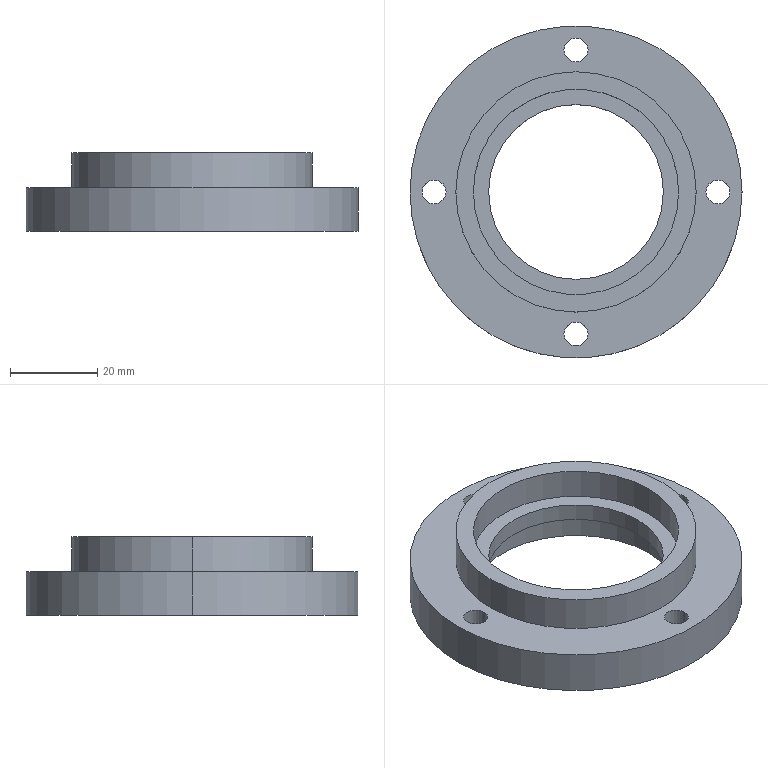Part | SolidWorks | features ICE 4, Extrusion 1, HoleWzd 1 | 1 solid | 35 faces | box 76 x 76 x 18 mm | volume 32922 mm3 | cylinder 26 | plane 9 | commonest cylinder face diameters 5.5 x8 10 x8 47 x4 40 x2 55 x2 76 x2
STEP:
#1=CARTESIAN_POINT('',(5.,32.5,5.4));
#2=VERTEX_POINT('',#1);
#3=CARTESIAN_POINT('',(-5.,32.5,5.4));
#4=VERTEX_POINT('',#3);
#5=CARTESIAN_POINT('',(0.,32.5,5.4));
#6=DIRECTION('',(0.,0.,-1.));
#7=DIRECTION('',(-1.,0.,0.));
#8=AXIS2_PLACEMENT_3D('',#5,#6,#7);
#9=CIRCLE('',#8,5.);
#10=EDGE_CURVE('',#2,#4,#9,.T.);
#11=ORIENTED_EDGE('',*,*,#10,.F.);
#12=CARTESIAN_POINT('',(5.,32.5,0.));
#13=VERTEX_POINT('',#12);
#14=CARTESIAN_POINT('',(5.,32.5,0.));
#15=DIRECTION('',(0.,0.,-1.));
#16=VECTOR('',#15,1000.);
#17=LINE('',#14,#16);
#18=EDGE_CURVE('',#2,#13,#17,.T.);
#19=ORIENTED_EDGE('',*,*,#18,.T.);
#20=CARTESIAN_POINT('',(-5.,32.5,0.));
#21=VERTEX_POINT('',#20);
#22=CARTESIAN_POINT('',(0.,32.5,0.));
#23=DIRECTION('',(0.,0.,-1.));
#24=DIRECTION('',(-1.,0.,0.));
#25=AXIS2_PLACEMENT_3D('',#22,#23,#24);
#26=CIRCLE('',#25,5.);
#27=EDGE_CURVE('',#13,#21,#26,.T.);
#28=ORIENTED_EDGE('',*,*,#27,.T.);
#29=CARTESIAN_POINT('',(-5.,32.5,0.));
#30=DIRECTION('',(0.,0.,-1.));
#31=VECTOR('',#30,1000.);
#32=LINE('',#29,#31);
#33=EDGE_CURVE('',#4,#21,#32,.T.);
#34=ORIENTED_EDGE('',*,*,#33,.F.);
#35=EDGE_LOOP('',(#11,#19,#28,#34));
#36=FACE_OUTER_BOUND('',#35,.T.);
#37=CARTESIAN_POINT('',(0.,32.5,0.));
#38=DIRECTION('',(0.,0.,-1.));
#39=DIRECTION('',(-1.,0.,0.));
#40=AXIS2_PLACEMENT_3D('',#37,#38,#39);
#41=CYLINDRICAL_SURFACE('',#40,5.);
#42=ADVANCED_FACE('',(#36),#41,.F.);
#43=CARTESIAN_POINT('',(-2.75,32.5,10.));
#44=VERTEX_POINT('',#43);
#45=CARTESIAN_POINT('',(2.75,32.5,10.));
#46=VERTEX_POINT('',#45);
#47=CARTESIAN_POINT('',(0.,32.5,10.));
#48=DIRECTION('',(0.,0.,1.));
#49=DIRECTION('',(1.,0.,0.));
#50=AXIS2_PLACEMENT_3D('',#47,#48,#49);
#51=CIRCLE('',#50,2.75);
#52=EDGE_CURVE('',#44,#46,#51,.T.);
#53=ORIENTED_EDGE('',*,*,#52,.T.);
#54=CARTESIAN_POINT('',(2.75,32.5,5.4));
#55=VERTEX_POINT('',#54);
#56=CARTESIAN_POINT('',(2.75,32.5,0.));
#57=DIRECTION('',(0.,0.,-1.));
#58=VECTOR('',#57,1000.);
#59=LINE('',#56,#58);
#60=EDGE_CURVE('',#46,#55,#59,.T.);
#61=ORIENTED_EDGE('',*,*,#60,.T.);
#62=CARTESIAN_POINT('',(-2.75,32.5,5.4));
#63=VERTEX_POINT('',#62);
#64=CARTESIAN_POINT('',(0.,32.5,5.4));
#65=DIRECTION('',(0.,0.,-1.));
#66=DIRECTION('',(-1.,0.,0.));
#67=AXIS2_PLACEMENT_3D('',#64,#65,#66);
#68=CIRCLE('',#67,2.75);
#69=EDGE_CURVE('',#55,#63,#68,.T.);
#70=ORIENTED_EDGE('',*,*,#69,.T.);
#71=CARTESIAN_POINT('',(-2.75,32.5,0.));
#72=DIRECTION('',(0.,0.,-1.));
#73=VECTOR('',#72,1000.);
#74=LINE('',#71,#73);
#75=EDGE_CURVE('',#44,#63,#74,.T.);
#76=ORIENTED_EDGE('',*,*,#75,.F.);
#77=EDGE_LOOP('',(#53,#61,#70,#76));
#78=FACE_OUTER_BOUND('',#77,.T.);
#79=CARTESIAN_POINT('',(0.,32.5,0.));
#80=DIRECTION('',(0.,0.,-1.));
#81=DIRECTION('',(-1.,0.,0.));
#82=AXIS2_PLACEMENT_3D('',#79,#80,#81);
#83=CYLINDRICAL_SURFACE('',#82,2.75);
#84=ADVANCED_FACE('',(#78),#83,.F.);
#85=CARTESIAN_POINT('',(37.5,0.,5.4));
#86=VERTEX_POINT('',#85);
#87=CARTESIAN_POINT('',(27.5,0.,5.4));
#88=VERTEX_POINT('',#87);
#89=CARTESIAN_POINT('',(32.5,0.,5.4));
#90=DIRECTION('',(0.,0.,-1.));
#91=DIRECTION('',(-1.,0.,0.));
#92=AXIS2_PLACEMENT_3D('',#89,#90,#91);
#93=CIRCLE('',#92,5.);
#94=EDGE_CURVE('',#86,#88,#93,.T.);
#95=ORIENTED_EDGE('',*,*,#94,.F.);
#96=CARTESIAN_POINT('',(37.5,0.,0.));
#97=VERTEX_POINT('',#96);
#98=CARTESIAN_POINT('',(37.5,0.,0.));
#99=DIRECTION('',(0.,0.,-1.));
#100=VECTOR('',#99,1000.);
#101=LINE('',#98,#100);
#102=EDGE_CURVE('',#86,#97,#101,.T.);
#103=ORIENTED_EDGE('',*,*,#102,.T.);
#104=CARTESIAN_POINT('',(27.5,0.,0.));
#105=VERTEX_POINT('',#104);
#106=CARTESIAN_POINT('',(32.5,0.,0.));
#107=DIRECTION('',(0.,0.,-1.));
#108=DIRECTION('',(-1.,0.,0.));
#109=AXIS2_PLACEMENT_3D('',#106,#107,#108);
#110=CIRCLE('',#109,5.);
#111=EDGE_CURVE('',#97,#105,#110,.T.);
#112=ORIENTED_EDGE('',*,*,#111,.T.);
#113=CARTESIAN_POINT('',(27.5,0.,0.));
#114=DIRECTION('',(0.,0.,-1.));
#115=VECTOR('',#114,1000.);
#116=LINE('',#113,#115);
#117=EDGE_CURVE('',#88,#105,#116,.T.);
#118=ORIENTED_EDGE('',*,*,#117,.F.);
#119=EDGE_LOOP('',(#95,#103,#112,#118));
#120=FACE_OUTER_BOUND('',#119,.T.);
#121=CARTESIAN_POINT('',(32.5,0.,0.));
#122=DIRECTION('',(0.,0.,-1.));
#123=DIRECTION('',(-1.,0.,0.));
#124=AXIS2_PLACEMENT_3D('',#121,#122,#123);
#125=CYLINDRICAL_SURFACE('',#124,5.);
#126=ADVANCED_FACE('',(#120),#125,.F.);
#127=CARTESIAN_POINT('',(29.75,0.,10.));
#128=VERTEX_POINT('',#127);
#129=CARTESIAN_POINT('',(35.25,0.,10.));
#130=VERTEX_POINT('',#129);
#131=CARTESIAN_POINT('',(32.5,0.,10.));
#132=DIRECTION('',(0.,0.,1.));
#133=DIRECTION('',(1.,0.,0.));
#134=AXIS2_PLACEMENT_3D('',#131,#132,#133);
#135=CIRCLE('',#134,2.75);
#136=EDGE_CURVE('',#128,#130,#135,.T.);
#137=ORIENTED_EDGE('',*,*,#136,.T.);
#138=CARTESIAN_POINT('',(35.25,0.,5.4));
#139=VERTEX_POINT('',#138);
#140=CARTESIAN_POINT('',(35.25,0.,0.));
#141=DIRECTION('',(0.,0.,-1.));
#142=VECTOR('',#141,1000.);
#143=LINE('',#140,#142);
#144=EDGE_CURVE('',#130,#139,#143,.T.);
#145=ORIENTED_EDGE('',*,*,#144,.T.);
#146=CARTESIAN_POINT('',(29.75,0.,5.4));
#147=VERTEX_POINT('',#146);
#148=CARTESIAN_POINT('',(32.5,0.,5.4));
#149=DIRECTION('',(0.,0.,-1.));
#150=DIRECTION('',(-1.,0.,0.));
#151=AXIS2_PLACEMENT_3D('',#148,#149,#150);
#152=CIRCLE('',#151,2.75);
#153=EDGE_CURVE('',#139,#147,#152,.T.);
#154=ORIENTED_EDGE('',*,*,#153,.T.);
#155=CARTESIAN_POINT('',(29.75,0.,0.));
#156=DIRECTION('',(0.,0.,-1.));
#157=VECTOR('',#156,1000.);
#158=LINE('',#155,#157);
#159=EDGE_CURVE('',#128,#147,#158,.T.);
#160=ORIENTED_EDGE('',*,*,#159,.F.);
#161=EDGE_LOOP('',(#137,#145,#154,#160));
#162=FACE_OUTER_BOUND('',#161,.T.);
#163=CARTESIAN_POINT('',(32.5,0.,0.));
#164=DIRECTION('',(0.,0.,-1.));
#165=DIRECTION('',(-1.,0.,0.));
#166=AXIS2_PLACEMENT_3D('',#163,#164,#165);
#167=CYLINDRICAL_SURFACE('',#166,2.75);
#168=ADVANCED_FACE('',(#162),#167,.F.);
#169=CARTESIAN_POINT('',(5.,-32.5,5.4));
#170=VERTEX_POINT('',#169);
#171=CARTESIAN_POINT('',(-5.,-32.5,5.4));
#172=VERTEX_POINT('',#171);
#173=CARTESIAN_POINT('',(0.,-32.5,5.4));
#174=DIRECTION('',(0.,0.,-1.));
#175=DIRECTION('',(-1.,0.,0.));
#176=AXIS2_PLACEMENT_3D('',#173,#174,#175);
#177=CIRCLE('',#176,5.);
#178=EDGE_CURVE('',#170,#172,#177,.T.);
#179=ORIENTED_EDGE('',*,*,#178,.F.);
#180=CARTESIAN_POINT('',(5.,-32.5,0.));
#181=VERTEX_POINT('',#180);
#182=CARTESIAN_POINT('',(5.,-32.5,0.));
#183=DIRECTION('',(0.,0.,-1.));
#184=VECTOR('',#183,1000.);
#185=LINE('',#182,#184);
#186=EDGE_CURVE('',#170,#181,#185,.T.);
#187=ORIENTED_EDGE('',*,*,#186,.T.);
#188=CARTESIAN_POINT('',(-5.,-32.5,0.));
#189=VERTEX_POINT('',#188);
#190=CARTESIAN_POINT('',(0.,-32.5,0.));
#191=DIRECTION('',(0.,0.,-1.));
#192=DIRECTION('',(-1.,0.,0.));
#193=AXIS2_PLACEMENT_3D('',#190,#191,#192);
#194=CIRCLE('',#193,5.);
#195=EDGE_CURVE('',#181,#189,#194,.T.);
#196=ORIENTED_EDGE('',*,*,#195,.T.);
#197=CARTESIAN_POINT('',(-5.,-32.5,0.));
#198=DIRECTION('',(0.,0.,-1.));
#199=VECTOR('',#198,1000.);
#200=LINE('',#197,#199);
#201=EDGE_CURVE('',#172,#189,#200,.T.);
#202=ORIENTED_EDGE('',*,*,#201,.F.);
#203=EDGE_LOOP('',(#179,#187,#196,#202));
#204=FACE_OUTER_BOUND('',#203,.T.);
#205=CARTESIAN_POINT('',(0.,-32.5,0.));
#206=DIRECTION('',(0.,0.,-1.));
#207=DIRECTION('',(-1.,0.,0.));
#208=AXIS2_PLACEMENT_3D('',#205,#206,#207);
#209=CYLINDRICAL_SURFACE('',#208,5.);
#210=ADVANCED_FACE('',(#204),#209,.F.);
#211=CARTESIAN_POINT('',(-2.75,-32.5,10.));
#212=VERTEX_POINT('',#211);
#213=CARTESIAN_POINT('',(2.75,-32.5,10.));
#214=VERTEX_POINT('',#213);
#215=CARTESIAN_POINT('',(0.,-32.5,10.));
#216=DIRECTION('',(0.,0.,1.));
#217=DIRECTION('',(1.,0.,0.));
#218=AXIS2_PLACEMENT_3D('',#215,#216,#217);
#219=CIRCLE('',#218,2.75);
#220=EDGE_CURVE('',#212,#214,#219,.T.);
#221=ORIENTED_EDGE('',*,*,#220,.T.);
#222=CARTESIAN_POINT('',(2.75,-32.5,5.4));
#223=VERTEX_POINT('',#222);
#224=CARTESIAN_POINT('',(2.75,-32.5,0.));
#225=DIRECTION('',(0.,0.,-1.));
#226=VECTOR('',#225,1000.);
#227=LINE('',#224,#226);
#228=EDGE_CURVE('',#214,#223,#227,.T.);
#229=ORIENTED_EDGE('',*,*,#228,.T.);
#230=CARTESIAN_POINT('',(-2.75,-32.5,5.4));
#231=VERTEX_POINT('',#230);
#232=CARTESIAN_POINT('',(0.,-32.5,5.4));
#233=DIRECTION('',(0.,0.,-1.));
#234=DIRECTION('',(-1.,0.,0.));
#235=AXIS2_PLACEMENT_3D('',#232,#233,#234);
#236=CIRCLE('',#235,2.75);
#237=EDGE_CURVE('',#223,#231,#236,.T.);
#238=ORIENTED_EDGE('',*,*,#237,.T.);
#239=CARTESIAN_POINT('',(-2.75,-32.5,0.));
#240=DIRECTION('',(0.,0.,-1.));
#241=VECTOR('',#240,1000.);
#242=LINE('',#239,#241);
#243=EDGE_CURVE('',#212,#231,#242,.T.);
#244=ORIENTED_EDGE('',*,*,#243,.F.);
#245=EDGE_LOOP('',(#221,#229,#238,#244));
#246=FACE_OUTER_BOUND('',#245,.T.);
#247=CARTESIAN_POINT('',(0.,-32.5,0.));
#248=DIRECTION('',(0.,0.,-1.));
#249=DIRECTION('',(-1.,0.,0.));
#250=AXIS2_PLACEMENT_3D('',#247,#248,#249);
#251=CYLINDRICAL_SURFACE('',#250,2.75);
#252=ADVANCED_FACE('',(#246),#251,.F.);
#253=CARTESIAN_POINT('',(-27.5,0.,5.4));
#254=VERTEX_POINT('',#253);
#255=CARTESIAN_POINT('',(-37.5,0.,5.4));
#256=VERTEX_POINT('',#255);
#257=CARTESIAN_POINT('',(-32.5,0.,5.4));
#258=DIRECTION('',(0.,0.,-1.));
#259=DIRECTION('',(-1.,0.,0.));
#260=AXIS2_PLACEMENT_3D('',#257,#258,#259);
#261=CIRCLE('',#260,5.);
#262=EDGE_CURVE('',#254,#256,#261,.T.);
#263=ORIENTED_EDGE('',*,*,#262,.F.);
#264=CARTESIAN_POINT('',(-27.5,0.,0.));
#265=VERTEX_POINT('',#264);
#266=CARTESIAN_POINT('',(-27.5,0.,0.));
#267=DIRECTION('',(0.,0.,-1.));
#268=VECTOR('',#267,1000.);
#269=LINE('',#266,#268);
#270=EDGE_CURVE('',#254,#265,#269,.T.);
#271=ORIENTED_EDGE('',*,*,#270,.T.);
#272=CARTESIAN_POINT('',(-37.5,0.,0.));
#273=VERTEX_POINT('',#272);
#274=CARTESIAN_POINT('',(-32.5,0.,0.));
#275=DIRECTION('',(0.,0.,-1.));
#276=DIRECTION('',(-1.,0.,0.));
#277=AXIS2_PLACEMENT_3D('',#274,#275,#276);
#278=CIRCLE('',#277,5.);
#279=EDGE_CURVE('',#265,#273,#278,.T.);
#280=ORIENTED_EDGE('',*,*,#279,.T.);
#281=CARTESIAN_POINT('',(-37.5,0.,0.));
#282=DIRECTION('',(0.,0.,-1.));
#283=VECTOR('',#282,1000.);
#284=LINE('',#281,#283);
#285=EDGE_CURVE('',#256,#273,#284,.T.);
#286=ORIENTED_EDGE('',*,*,#285,.F.);
#287=EDGE_LOOP('',(#263,#271,#280,#286));
#288=FACE_OUTER_BOUND('',#287,.T.);
#289=CARTESIAN_POINT('',(-32.5,0.,0.));
#290=DIRECTION('',(0.,0.,-1.));
#291=DIRECTION('',(-1.,0.,0.));
#292=AXIS2_PLACEMENT_3D('',#289,#290,#291);
#293=CYLINDRICAL_SURFACE('',#292,5.);
#294=ADVANCED_FACE('',(#288),#293,.F.);
#295=CARTESIAN_POINT('',(-35.25,0.,10.));
#296=VERTEX_POINT('',#295);
#297=CARTESIAN_POINT('',(-29.75,0.,10.));
#298=VERTEX_POINT('',#297);
#299=CARTESIAN_POINT('',(-32.5,0.,10.));
#300=DIRECTION('',(0.,0.,1.));
#301=DIRECTION('',(1.,0.,0.));
#302=AXIS2_PLACEMENT_3D('',#299,#300,#301);
#303=CIRCLE('',#302,2.75);
#304=EDGE_CURVE('',#296,#298,#303,.T.);
#305=ORIENTED_EDGE('',*,*,#304,.T.);
#306=CARTESIAN_POINT('',(-29.75,0.,5.4));
#307=VERTEX_POINT('',#306);
#308=CARTESIAN_POINT('',(-29.75,0.,0.));
#309=DIRECTION('',(0.,0.,-1.));
#310=VECTOR('',#309,1000.);
#311=LINE('',#308,#310);
#312=EDGE_CURVE('',#298,#307,#311,.T.);
#313=ORIENTED_EDGE('',*,*,#312,.T.);
#314=CARTESIAN_POINT('',(-35.25,0.,5.4));
#315=VERTEX_POINT('',#314);
#316=CARTESIAN_POINT('',(-32.5,0.,5.4));
#317=DIRECTION('',(0.,0.,-1.));
#318=DIRECTION('',(-1.,0.,0.));
#319=AXIS2_PLACEMENT_3D('',#316,#317,#318);
#320=CIRCLE('',#319,2.75);
#321=EDGE_CURVE('',#307,#315,#320,.T.);
#322=ORIENTED_EDGE('',*,*,#321,.T.);
#323=CARTESIAN_POINT('',(-35.25,0.,0.));
#324=DIRECTION('',(0.,0.,-1.));
#325=VECTOR('',#324,1000.);
#326=LINE('',#323,#325);
#327=EDGE_CURVE('',#296,#315,#326,.T.);
#328=ORIENTED_EDGE('',*,*,#327,.F.);
#329=EDGE_LOOP('',(#305,#313,#322,#328));
#330=FACE_OUTER_BOUND('',#329,.T.);
#331=CARTESIAN_POINT('',(-32.5,0.,0.));
#332=DIRECTION('',(0.,0.,-1.));
#333=DIRECTION('',(-1.,0.,0.));
#334=AXIS2_PLACEMENT_3D('',#331,#332,#333);
#335=CYLINDRICAL_SURFACE('',#334,2.75);
#336=ADVANCED_FACE('',(#330),#335,.F.);
#337=CARTESIAN_POINT('',(20.,0.,7.));
#338=VERTEX_POINT('',#337);
#339=CARTESIAN_POINT('',(-20.,0.,7.));
#340=VERTEX_POINT('',#339);
#341=CARTESIAN_POINT('',(0.,0.,7.));
#342=DIRECTION('',(0.,0.,-1.));
#343=DIRECTION('',(-1.,0.,0.));
#344=AXIS2_PLACEMENT_3D('',#341,#342,#343);
#345=CIRCLE('',#344,20.);
#346=EDGE_CURVE('',#338,#340,#345,.T.);
#347=ORIENTED_EDGE('',*,*,#346,.T.);
#348=CARTESIAN_POINT('',(-20.,0.,11.));
#349=VERTEX_POINT('',#348);
#350=CARTESIAN_POINT('',(-20.,0.,0.));
#351=DIRECTION('',(0.,0.,1.));
#352=VECTOR('',#351,1000.);
#353=LINE('',#350,#352);
#354=EDGE_CURVE('',#340,#349,#353,.T.);
#355=ORIENTED_EDGE('',*,*,#354,.T.);
#356=CARTESIAN_POINT('',(20.,0.,11.));
#357=VERTEX_POINT('',#356);
#358=CARTESIAN_POINT('',(0.,0.,11.));
#359=DIRECTION('',(0.,0.,1.));
#360=DIRECTION('',(1.,0.,0.));
#361=AXIS2_PLACEMENT_3D('',#358,#359,#360);
#362=CIRCLE('',#361,20.);
#363=EDGE_CURVE('',#349,#357,#362,.T.);
#364=ORIENTED_EDGE('',*,*,#363,.T.);
#365=CARTESIAN_POINT('',(20.,0.,0.));
#366=DIRECTION('',(0.,0.,1.));
#367=VECTOR('',#366,1000.);
#368=LINE('',#365,#367);
#369=EDGE_CURVE('',#338,#357,#368,.T.);
#370=ORIENTED_EDGE('',*,*,#369,.F.);
#371=EDGE_LOOP('',(#347,#355,#364,#370));
#372=FACE_OUTER_BOUND('',#371,.T.);
#373=CARTESIAN_POINT('',(0.,0.,0.));
#374=DIRECTION('',(0.,0.,1.));
#375=DIRECTION('',(1.,0.,0.));
#376=AXIS2_PLACEMENT_3D('',#373,#374,#375);
#377=CYLINDRICAL_SURFACE('',#376,20.);
#378=ADVANCED_FACE('',(#372),#377,.F.);
#379=CARTESIAN_POINT('',(23.5,0.,7.));
#380=VERTEX_POINT('',#379);
#381=CARTESIAN_POINT('',(-23.5,0.,7.));
#382=VERTEX_POINT('',#381);
#383=CARTESIAN_POINT('',(0.,0.,7.));
#384=DIRECTION('',(0.,0.,-1.));
#385=DIRECTION('',(-1.,0.,0.));
#386=AXIS2_PLACEMENT_3D('',#383,#384,#385);
#387=CIRCLE('',#386,23.5);
#388=EDGE_CURVE('',#380,#382,#387,.T.);
#389=ORIENTED_EDGE('',*,*,#388,.F.);
#390=CARTESIAN_POINT('',(23.5,0.,0.));
#391=VERTEX_POINT('',#390);
#392=CARTESIAN_POINT('',(23.5,0.,7.));
#393=DIRECTION('',(0.,0.,-1.));
#394=VECTOR('',#393,1000.);
#395=LINE('',#392,#394);
#396=EDGE_CURVE('',#380,#391,#395,.T.);
#397=ORIENTED_EDGE('',*,*,#396,.T.);
#398=CARTESIAN_POINT('',(-23.5,0.,0.));
#399=VERTEX_POINT('',#398);
#400=CARTESIAN_POINT('',(0.,0.,0.));
#401=DIRECTION('',(0.,0.,-1.));
#402=DIRECTION('',(-1.,0.,0.));
#403=AXIS2_PLACEMENT_3D('',#400,#401,#402);
#404=CIRCLE('',#403,23.5);
#405=EDGE_CURVE('',#391,#399,#404,.T.);
#406=ORIENTED_EDGE('',*,*,#405,.T.);
#407=CARTESIAN_POINT('',(-23.5,0.,7.));
#408=DIRECTION('',(0.,0.,-1.));
#409=VECTOR('',#408,1000.);
#410=LINE('',#407,#409);
#411=EDGE_CURVE('',#382,#399,#410,.T.);
#412=ORIENTED_EDGE('',*,*,#411,.F.);
#413=EDGE_LOOP('',(#389,#397,#406,#412));
#414=FACE_OUTER_BOUND('',#413,.T.);
#415=CARTESIAN_POINT('',(0.,0.,7.));
#416=DIRECTION('',(0.,0.,-1.));
#417=DIRECTION('',(-1.,0.,0.));
#418=AXIS2_PLACEMENT_3D('',#415,#416,#417);
#419=CYLINDRICAL_SURFACE('',#418,23.5);
#420=ADVANCED_FACE('',(#414),#419,.F.);
#421=CARTESIAN_POINT('',(-23.5,0.,11.));
#422=VERTEX_POINT('',#421);
#423=CARTESIAN_POINT('',(23.5,0.,11.));
#424=VERTEX_POINT('',#423);
#425=CARTESIAN_POINT('',(0.,0.,11.));
#426=DIRECTION('',(0.,0.,1.));
#427=DIRECTION('',(1.,0.,0.));
#428=AXIS2_PLACEMENT_3D('',#425,#426,#427);
#429=CIRCLE('',#428,23.5);
#430=EDGE_CURVE('',#422,#424,#429,.T.);
#431=ORIENTED_EDGE('',*,*,#430,.F.);
#432=CARTESIAN_POINT('',(-23.5,0.,18.));
#433=VERTEX_POINT('',#432);
#434=CARTESIAN_POINT('',(-23.5,0.,11.));
#435=DIRECTION('',(0.,0.,1.));
#436=VECTOR('',#435,1000.);
#437=LINE('',#434,#436);
#438=EDGE_CURVE('',#422,#433,#437,.T.);
#439=ORIENTED_EDGE('',*,*,#438,.T.);
#440=CARTESIAN_POINT('',(23.5,0.,18.));
#441=VERTEX_POINT('',#440);
#442=CARTESIAN_POINT('',(0.,0.,18.));
#443=DIRECTION('',(0.,0.,1.));
#444=DIRECTION('',(1.,0.,0.));
#445=AXIS2_PLACEMENT_3D('',#442,#443,#444);
#446=CIRCLE('',#445,23.5);
#447=EDGE_CURVE('',#433,#441,#446,.T.);
#448=ORIENTED_EDGE('',*,*,#447,.T.);
#449=CARTESIAN_POINT('',(23.5,0.,11.));
#450=DIRECTION('',(0.,0.,1.));
#451=VECTOR('',#450,1000.);
#452=LINE('',#449,#451);
#453=EDGE_CURVE('',#424,#441,#452,.T.);
#454=ORIENTED_EDGE('',*,*,#453,.F.);
#455=EDGE_LOOP('',(#431,#439,#448,#454));
#456=FACE_OUTER_BOUND('',#455,.T.);
#457=CARTESIAN_POINT('',(0.,0.,11.));
#458=DIRECTION('',(0.,0.,1.));
#459=DIRECTION('',(1.,0.,0.));
#460=AXIS2_PLACEMENT_3D('',#457,#458,#459);
#461=CYLINDRICAL_SURFACE('',#460,23.5);
#462=ADVANCED_FACE('',(#456),#461,.F.);
#463=CARTESIAN_POINT('',(27.5,0.,18.));
#464=VERTEX_POINT('',#463);
#465=CARTESIAN_POINT('',(-27.5,0.,18.));
#466=VERTEX_POINT('',#465);
#467=CARTESIAN_POINT('',(0.,0.,18.));
#468=DIRECTION('',(0.,0.,1.));
#469=DIRECTION('',(1.,0.,0.));
#470=AXIS2_PLACEMENT_3D('',#467,#468,#469);
#471=CIRCLE('',#470,27.5);
#472=EDGE_CURVE('',#464,#466,#471,.T.);
#473=ORIENTED_EDGE('',*,*,#472,.F.);
#474=CARTESIAN_POINT('',(27.5,0.,10.));
#475=VERTEX_POINT('',#474);
#476=CARTESIAN_POINT('',(27.5,0.,18.));
#477=DIRECTION('',(0.,0.,-1.));
#478=VECTOR('',#477,1000.);
#479=LINE('',#476,#478);
#480=EDGE_CURVE('',#464,#475,#479,.T.);
#481=ORIENTED_EDGE('',*,*,#480,.T.);
#482=CARTESIAN_POINT('',(-27.5,0.,10.));
#483=VERTEX_POINT('',#482);
#484=CARTESIAN_POINT('',(0.,0.,10.));
#485=DIRECTION('',(0.,0.,1.));
#486=DIRECTION('',(1.,0.,0.));
#487=AXIS2_PLACEMENT_3D('',#484,#485,#486);
#488=CIRCLE('',#487,27.5);
#489=EDGE_CURVE('',#475,#483,#488,.T.);
#490=ORIENTED_EDGE('',*,*,#489,.T.);
#491=CARTESIAN_POINT('',(-27.5,0.,18.));
#492=DIRECTION('',(0.,0.,-1.));
#493=VECTOR('',#492,1000.);
#494=LINE('',#491,#493);
#495=EDGE_CURVE('',#466,#483,#494,.T.);
#496=ORIENTED_EDGE('',*,*,#495,.F.);
#497=EDGE_LOOP('',(#473,#481,#490,#496));
#498=FACE_OUTER_BOUND('',#497,.T.);
#499=CARTESIAN_POINT('',(0.,0.,18.));
#500=DIRECTION('',(0.,0.,-1.));
#501=DIRECTION('',(-1.,0.,0.));
#502=AXIS2_PLACEMENT_3D('',#499,#500,#501);
#503=CYLINDRICAL_SURFACE('',#502,27.5);
#504=ADVANCED_FACE('',(#498),#503,.T.);
#505=CARTESIAN_POINT('',(38.,0.,10.));
#506=VERTEX_POINT('',#505);
#507=CARTESIAN_POINT('',(-38.,0.,10.));
#508=VERTEX_POINT('',#507);
#509=CARTESIAN_POINT('',(0.,0.,10.));
#510=DIRECTION('',(0.,0.,1.));
#511=DIRECTION('',(1.,0.,0.));
#512=AXIS2_PLACEMENT_3D('',#509,#510,#511);
#513=CIRCLE('',#512,38.);
#514=EDGE_CURVE('',#506,#508,#513,.T.);
#515=ORIENTED_EDGE('',*,*,#514,.F.);
#516=CARTESIAN_POINT('',(38.,0.,0.));
#517=VERTEX_POINT('',#516);
#518=CARTESIAN_POINT('',(38.,0.,10.));
#519=DIRECTION('',(0.,0.,-1.));
#520=VECTOR('',#519,1000.);
#521=LINE('',#518,#520);
#522=EDGE_CURVE('',#506,#517,#521,.T.);
#523=ORIENTED_EDGE('',*,*,#522,.T.);
#524=CARTESIAN_POINT('',(-38.,0.,0.));
#525=VERTEX_POINT('',#524);
#526=CARTESIAN_POINT('',(0.,0.,0.));
#527=DIRECTION('',(0.,0.,1.));
#528=DIRECTION('',(1.,0.,0.));
#529=AXIS2_PLACEMENT_3D('',#526,#527,#528);
#530=CIRCLE('',#529,38.);
#531=EDGE_CURVE('',#517,#525,#530,.T.);
#532=ORIENTED_EDGE('',*,*,#531,.T.);
#533=CARTESIAN_POINT('',(-38.,0.,10.));
#534=DIRECTION('',(0.,0.,-1.));
#535=VECTOR('',#534,1000.);
#536=LINE('',#533,#535);
#537=EDGE_CURVE('',#508,#525,#536,.T.);
#538=ORIENTED_EDGE('',*,*,#537,.F.);
#539=EDGE_LOOP('',(#515,#523,#532,#538));
#540=FACE_OUTER_BOUND('',#539,.T.);
#541=CARTESIAN_POINT('',(0.,0.,10.));
#542=DIRECTION('',(0.,0.,-1.));
#543=DIRECTION('',(-1.,0.,0.));
#544=AXIS2_PLACEMENT_3D('',#541,#542,#543);
#545=CYLINDRICAL_SURFACE('',#544,38.);
#546=ADVANCED_FACE('',(#540),#545,.T.);
#547=ORIENTED_EDGE('',*,*,#522,.F.);
#548=CARTESIAN_POINT('',(0.,0.,10.));
#549=DIRECTION('',(0.,0.,1.));
#550=DIRECTION('',(1.,0.,0.));
#551=AXIS2_PLACEMENT_3D('',#548,#549,#550);
#552=CIRCLE('',#551,38.);
#553=EDGE_CURVE('',#508,#506,#552,.T.);
#554=ORIENTED_EDGE('',*,*,#553,.F.);
#555=ORIENTED_EDGE('',*,*,#537,.T.);
#556=CARTESIAN_POINT('',(0.,0.,0.));
#557=DIRECTION('',(0.,0.,1.));
#558=DIRECTION('',(1.,0.,0.));
#559=AXIS2_PLACEMENT_3D('',#556,#557,#558);
#560=CIRCLE('',#559,38.);
#561=EDGE_CURVE('',#525,#517,#560,.T.);
#562=ORIENTED_EDGE('',*,*,#561,.T.);
#563=EDGE_LOOP('',(#547,#554,#555,#562));
#564=FACE_OUTER_BOUND('',#563,.T.);
#565=CARTESIAN_POINT('',(0.,0.,10.));
#566=DIRECTION('',(0.,0.,-1.));
#567=DIRECTION('',(-1.,0.,0.));
#568=AXIS2_PLACEMENT_3D('',#565,#566,#567);
#569=CYLINDRICAL_SURFACE('',#568,38.);
#570=ADVANCED_FACE('',(#564),#569,.T.);
#571=ORIENTED_EDGE('',*,*,#52,.F.);
#572=CARTESIAN_POINT('',(0.,32.5,10.));
#573=DIRECTION('',(0.,0.,1.));
#574=DIRECTION('',(1.,0.,0.));
#575=AXIS2_PLACEMENT_3D('',#572,#573,#574);
#576=CIRCLE('',#575,2.75);
#577=EDGE_CURVE('',#46,#44,#576,.T.);
#578=ORIENTED_EDGE('',*,*,#577,.F.);
#579=EDGE_LOOP('',(#571,#578));
#580=FACE_BOUND('',#579,.T.);
#581=ORIENTED_EDGE('',*,*,#136,.F.);
#582=CARTESIAN_POINT('',(32.5,0.,10.));
#583=DIRECTION('',(0.,0.,1.));
#584=DIRECTION('',(1.,0.,0.));
#585=AXIS2_PLACEMENT_3D('',#582,#583,#584);
#586=CIRCLE('',#585,2.75);
#587=EDGE_CURVE('',#130,#128,#586,.T.);
#588=ORIENTED_EDGE('',*,*,#587,.F.);
#589=EDGE_LOOP('',(#581,#588));
#590=FACE_BOUND('',#589,.T.);
#591=ORIENTED_EDGE('',*,*,#220,.F.);
#592=CARTESIAN_POINT('',(0.,-32.5,10.));
#593=DIRECTION('',(0.,0.,1.));
#594=DIRECTION('',(1.,0.,0.));
#595=AXIS2_PLACEMENT_3D('',#592,#593,#594);
#596=CIRCLE('',#595,2.75);
#597=EDGE_CURVE('',#214,#212,#596,.T.);
#598=ORIENTED_EDGE('',*,*,#597,.F.);
#599=EDGE_LOOP('',(#591,#598));
#600=FACE_BOUND('',#599,.T.);
#601=ORIENTED_EDGE('',*,*,#304,.F.);
#602=CARTESIAN_POINT('',(-32.5,0.,10.));
#603=DIRECTION('',(0.,0.,1.));
#604=DIRECTION('',(1.,0.,0.));
#605=AXIS2_PLACEMENT_3D('',#602,#603,#604);
#606=CIRCLE('',#605,2.75);
#607=EDGE_CURVE('',#298,#296,#606,.T.);
#608=ORIENTED_EDGE('',*,*,#607,.F.);
#609=EDGE_LOOP('',(#601,#608));
#610=FACE_BOUND('',#609,.T.);
#611=CARTESIAN_POINT('',(0.,0.,10.));
#612=DIRECTION('',(0.,0.,1.));
#613=DIRECTION('',(1.,0.,0.));
#614=AXIS2_PLACEMENT_3D('',#611,#612,#613);
#615=CIRCLE('',#614,27.5);
#616=EDGE_CURVE('',#483,#475,#615,.T.);
#617=ORIENTED_EDGE('',*,*,#616,.F.);
#618=ORIENTED_EDGE('',*,*,#489,.F.);
#619=EDGE_LOOP('',(#617,#618));
#620=FACE_BOUND('',#619,.T.);
#621=ORIENTED_EDGE('',*,*,#553,.T.);
#622=ORIENTED_EDGE('',*,*,#514,.T.);
#623=EDGE_LOOP('',(#621,#622));
#624=FACE_OUTER_BOUND('',#623,.T.);
#625=CARTESIAN_POINT('',(0.,0.,10.));
#626=DIRECTION('',(0.,0.,1.));
#627=DIRECTION('',(1.,0.,0.));
#628=AXIS2_PLACEMENT_3D('',#625,#626,#627);
#629=PLANE('',#628);
#630=ADVANCED_FACE('',(#580,#590,#600,#610,#620,#624),#629,.T.);
#631=CARTESIAN_POINT('',(0.,32.5,0.));
#632=DIRECTION('',(0.,0.,-1.));
#633=DIRECTION('',(-1.,0.,0.));
#634=AXIS2_PLACEMENT_3D('',#631,#632,#633);
#635=CIRCLE('',#634,5.);
#636=EDGE_CURVE('',#21,#13,#635,.T.);
#637=ORIENTED_EDGE('',*,*,#636,.F.);
#638=ORIENTED_EDGE('',*,*,#27,.F.);
#639=EDGE_LOOP('',(#637,#638));
#640=FACE_BOUND('',#639,.T.);
#641=CARTESIAN_POINT('',(32.5,0.,0.));
#642=DIRECTION('',(0.,0.,-1.));
#643=DIRECTION('',(-1.,0.,0.));
#644=AXIS2_PLACEMENT_3D('',#641,#642,#643);
#645=CIRCLE('',#644,5.);
#646=EDGE_CURVE('',#105,#97,#645,.T.);
#647=ORIENTED_EDGE('',*,*,#646,.F.);
#648=ORIENTED_EDGE('',*,*,#111,.F.);
#649=EDGE_LOOP('',(#647,#648));
#650=FACE_BOUND('',#649,.T.);
#651=CARTESIAN_POINT('',(0.,-32.5,0.));
#652=DIRECTION('',(0.,0.,-1.));
#653=DIRECTION('',(-1.,0.,0.));
#654=AXIS2_PLACEMENT_3D('',#651,#652,#653);
#655=CIRCLE('',#654,5.);
#656=EDGE_CURVE('',#189,#181,#655,.T.);
#657=ORIENTED_EDGE('',*,*,#656,.F.);
#658=ORIENTED_EDGE('',*,*,#195,.F.);
#659=EDGE_LOOP('',(#657,#658));
#660=FACE_BOUND('',#659,.T.);
#661=CARTESIAN_POINT('',(-32.5,0.,0.));
#662=DIRECTION('',(0.,0.,-1.));
#663=DIRECTION('',(-1.,0.,0.));
#664=AXIS2_PLACEMENT_3D('',#661,#662,#663);
#665=CIRCLE('',#664,5.);
#666=EDGE_CURVE('',#273,#265,#665,.T.);
#667=ORIENTED_EDGE('',*,*,#666,.F.);
#668=ORIENTED_EDGE('',*,*,#279,.F.);
#669=EDGE_LOOP('',(#667,#668));
#670=FACE_BOUND('',#669,.T.);
#671=CARTESIAN_POINT('',(0.,0.,0.));
#672=DIRECTION('',(0.,0.,-1.));
#673=DIRECTION('',(-1.,0.,0.));
#674=AXIS2_PLACEMENT_3D('',#671,#672,#673);
#675=CIRCLE('',#674,23.5);
#676=EDGE_CURVE('',#399,#391,#675,.T.);
#677=ORIENTED_EDGE('',*,*,#676,.F.);
#678=ORIENTED_EDGE('',*,*,#405,.F.);
#679=EDGE_LOOP('',(#677,#678));
#680=FACE_BOUND('',#679,.T.);
#681=ORIENTED_EDGE('',*,*,#561,.F.);
#682=ORIENTED_EDGE('',*,*,#531,.F.);
#683=EDGE_LOOP('',(#681,#682));
#684=FACE_OUTER_BOUND('',#683,.T.);
#685=CARTESIAN_POINT('',(0.,0.,0.));
#686=DIRECTION('',(0.,0.,1.));
#687=DIRECTION('',(1.,0.,0.));
#688=AXIS2_PLACEMENT_3D('',#685,#686,#687);
#689=PLANE('',#688);
#690=ADVANCED_FACE('',(#640,#650,#660,#670,#680,#684),#689,.F.);
#691=ORIENTED_EDGE('',*,*,#480,.F.);
#692=CARTESIAN_POINT('',(0.,0.,18.));
#693=DIRECTION('',(0.,0.,1.));
#694=DIRECTION('',(1.,0.,0.));
#695=AXIS2_PLACEMENT_3D('',#692,#693,#694);
#696=CIRCLE('',#695,27.5);
#697=EDGE_CURVE('',#466,#464,#696,.T.);
#698=ORIENTED_EDGE('',*,*,#697,.F.);
#699=ORIENTED_EDGE('',*,*,#495,.T.);
#700=ORIENTED_EDGE('',*,*,#616,.T.);
#701=EDGE_LOOP('',(#691,#698,#699,#700));
#702=FACE_OUTER_BOUND('',#701,.T.);
#703=CARTESIAN_POINT('',(0.,0.,18.));
#704=DIRECTION('',(0.,0.,-1.));
#705=DIRECTION('',(-1.,0.,0.));
#706=AXIS2_PLACEMENT_3D('',#703,#704,#705);
#707=CYLINDRICAL_SURFACE('',#706,27.5);
#708=ADVANCED_FACE('',(#702),#707,.T.);
#709=CARTESIAN_POINT('',(0.,0.,18.));
#710=DIRECTION('',(0.,0.,1.));
#711=DIRECTION('',(1.,0.,0.));
#712=AXIS2_PLACEMENT_3D('',#709,#710,#711);
#713=CIRCLE('',#712,23.5);
#714=EDGE_CURVE('',#441,#433,#713,.T.);
#715=ORIENTED_EDGE('',*,*,#714,.F.);
#716=ORIENTED_EDGE('',*,*,#447,.F.);
#717=EDGE_LOOP('',(#715,#716));
#718=FACE_BOUND('',#717,.T.);
#719=ORIENTED_EDGE('',*,*,#697,.T.);
#720=ORIENTED_EDGE('',*,*,#472,.T.);
#721=EDGE_LOOP('',(#719,#720));
#722=FACE_OUTER_BOUND('',#721,.T.);
#723=CARTESIAN_POINT('',(0.,0.,18.));
#724=DIRECTION('',(0.,0.,1.));
#725=DIRECTION('',(1.,0.,0.));
#726=AXIS2_PLACEMENT_3D('',#723,#724,#725);
#727=PLANE('',#726);
#728=ADVANCED_FACE('',(#718,#722),#727,.T.);
#729=ORIENTED_EDGE('',*,*,#438,.F.);
#730=CARTESIAN_POINT('',(0.,0.,11.));
#731=DIRECTION('',(0.,0.,1.));
#732=DIRECTION('',(1.,0.,0.));
#733=AXIS2_PLACEMENT_3D('',#730,#731,#732);
#734=CIRCLE('',#733,23.5);
#735=EDGE_CURVE('',#424,#422,#734,.T.);
#736=ORIENTED_EDGE('',*,*,#735,.F.);
#737=ORIENTED_EDGE('',*,*,#453,.T.);
#738=ORIENTED_EDGE('',*,*,#714,.T.);
#739=EDGE_LOOP('',(#729,#736,#737,#738));
#740=FACE_OUTER_BOUND('',#739,.T.);
#741=CARTESIAN_POINT('',(0.,0.,11.));
#742=DIRECTION('',(0.,0.,1.));
#743=DIRECTION('',(1.,0.,0.));
#744=AXIS2_PLACEMENT_3D('',#741,#742,#743);
#745=CYLINDRICAL_SURFACE('',#744,23.5);
#746=ADVANCED_FACE('',(#740),#745,.F.);
#747=CARTESIAN_POINT('',(0.,0.,11.));
#748=DIRECTION('',(0.,0.,1.));
#749=DIRECTION('',(1.,0.,0.));
#750=AXIS2_PLACEMENT_3D('',#747,#748,#749);
#751=CIRCLE('',#750,20.);
#752=EDGE_CURVE('',#357,#349,#751,.T.);
#753=ORIENTED_EDGE('',*,*,#752,.F.);
#754=ORIENTED_EDGE('',*,*,#363,.F.);
#755=EDGE_LOOP('',(#753,#754));
#756=FACE_BOUND('',#755,.T.);
#757=ORIENTED_EDGE('',*,*,#735,.T.);
#758=ORIENTED_EDGE('',*,*,#430,.T.);
#759=EDGE_LOOP('',(#757,#758));
#760=FACE_OUTER_BOUND('',#759,.T.);
#761=CARTESIAN_POINT('',(0.,0.,11.));
#762=DIRECTION('',(0.,0.,1.));
#763=DIRECTION('',(1.,0.,0.));
#764=AXIS2_PLACEMENT_3D('',#761,#762,#763);
#765=PLANE('',#764);
#766=ADVANCED_FACE('',(#756,#760),#765,.T.);
#767=ORIENTED_EDGE('',*,*,#396,.F.);
#768=CARTESIAN_POINT('',(0.,0.,7.));
#769=DIRECTION('',(0.,0.,-1.));
#770=DIRECTION('',(-1.,0.,0.));
#771=AXIS2_PLACEMENT_3D('',#768,#769,#770);
#772=CIRCLE('',#771,23.5);
#773=EDGE_CURVE('',#382,#380,#772,.T.);
#774=ORIENTED_EDGE('',*,*,#773,.F.);
#775=ORIENTED_EDGE('',*,*,#411,.T.);
#776=ORIENTED_EDGE('',*,*,#676,.T.);
#777=EDGE_LOOP('',(#767,#774,#775,#776));
#778=FACE_OUTER_BOUND('',#777,.T.);
#779=CARTESIAN_POINT('',(0.,0.,7.));
#780=DIRECTION('',(0.,0.,-1.));
#781=DIRECTION('',(-1.,0.,0.));
#782=AXIS2_PLACEMENT_3D('',#779,#780,#781);
#783=CYLINDRICAL_SURFACE('',#782,23.5);
#784=ADVANCED_FACE('',(#778),#783,.F.);
#785=ORIENTED_EDGE('',*,*,#346,.F.);
#786=CARTESIAN_POINT('',(0.,0.,7.));
#787=DIRECTION('',(0.,0.,-1.));
#788=DIRECTION('',(-1.,0.,0.));
#789=AXIS2_PLACEMENT_3D('',#786,#787,#788);
#790=CIRCLE('',#789,20.);
#791=EDGE_CURVE('',#340,#338,#790,.T.);
#792=ORIENTED_EDGE('',*,*,#791,.F.);
#793=EDGE_LOOP('',(#785,#792));
#794=FACE_BOUND('',#793,.T.);
#795=ORIENTED_EDGE('',*,*,#773,.T.);
#796=ORIENTED_EDGE('',*,*,#388,.T.);
#797=EDGE_LOOP('',(#795,#796));
#798=FACE_OUTER_BOUND('',#797,.T.);
#799=CARTESIAN_POINT('',(0.,0.,7.));
#800=DIRECTION('',(0.,0.,-1.));
#801=DIRECTION('',(-1.,0.,0.));
#802=AXIS2_PLACEMENT_3D('',#799,#800,#801);
#803=PLANE('',#802);
#804=ADVANCED_FACE('',(#794,#798),#803,.T.);
#805=ORIENTED_EDGE('',*,*,#354,.F.);
#806=ORIENTED_EDGE('',*,*,#791,.T.);
#807=ORIENTED_EDGE('',*,*,#369,.T.);
#808=ORIENTED_EDGE('',*,*,#752,.T.);
#809=EDGE_LOOP('',(#805,#806,#807,#808));
#810=FACE_OUTER_BOUND('',#809,.T.);
#811=CARTESIAN_POINT('',(0.,0.,0.));
#812=DIRECTION('',(0.,0.,1.));
#813=DIRECTION('',(1.,0.,0.));
#814=AXIS2_PLACEMENT_3D('',#811,#812,#813);
#815=CYLINDRICAL_SURFACE('',#814,20.);
#816=ADVANCED_FACE('',(#810),#815,.F.);
#817=ORIENTED_EDGE('',*,*,#312,.F.);
#818=ORIENTED_EDGE('',*,*,#607,.T.);
#819=ORIENTED_EDGE('',*,*,#327,.T.);
#820=CARTESIAN_POINT('',(-32.5,0.,5.4));
#821=DIRECTION('',(0.,0.,-1.));
#822=DIRECTION('',(-1.,0.,0.));
#823=AXIS2_PLACEMENT_3D('',#820,#821,#822);
#824=CIRCLE('',#823,2.75);
#825=EDGE_CURVE('',#315,#307,#824,.T.);
#826=ORIENTED_EDGE('',*,*,#825,.T.);
#827=EDGE_LOOP('',(#817,#818,#819,#826));
#828=FACE_OUTER_BOUND('',#827,.T.);
#829=CARTESIAN_POINT('',(-32.5,0.,0.));
#830=DIRECTION('',(0.,0.,-1.));
#831=DIRECTION('',(-1.,0.,0.));
#832=AXIS2_PLACEMENT_3D('',#829,#830,#831);
#833=CYLINDRICAL_SURFACE('',#832,2.75);
#834=ADVANCED_FACE('',(#828),#833,.F.);
#835=ORIENTED_EDGE('',*,*,#825,.F.);
#836=ORIENTED_EDGE('',*,*,#321,.F.);
#837=EDGE_LOOP('',(#835,#836));
#838=FACE_BOUND('',#837,.T.);
#839=CARTESIAN_POINT('',(-32.5,0.,5.4));
#840=DIRECTION('',(0.,0.,-1.));
#841=DIRECTION('',(-1.,0.,0.));
#842=AXIS2_PLACEMENT_3D('',#839,#840,#841);
#843=CIRCLE('',#842,5.);
#844=EDGE_CURVE('',#256,#254,#843,.T.);
#845=ORIENTED_EDGE('',*,*,#844,.T.);
#846=ORIENTED_EDGE('',*,*,#262,.T.);
#847=EDGE_LOOP('',(#845,#846));
#848=FACE_OUTER_BOUND('',#847,.T.);
#849=CARTESIAN_POINT('',(-29.75,0.,5.4));
#850=DIRECTION('',(0.,0.,1.));
#851=DIRECTION('',(1.,0.,0.));
#852=AXIS2_PLACEMENT_3D('',#849,#850,#851);
#853=PLANE('',#852);
#854=ADVANCED_FACE('',(#838,#848),#853,.F.);
#855=ORIENTED_EDGE('',*,*,#270,.F.);
#856=ORIENTED_EDGE('',*,*,#844,.F.);
#857=ORIENTED_EDGE('',*,*,#285,.T.);
#858=ORIENTED_EDGE('',*,*,#666,.T.);
#859=EDGE_LOOP('',(#855,#856,#857,#858));
#860=FACE_OUTER_BOUND('',#859,.T.);
#861=CARTESIAN_POINT('',(-32.5,0.,0.));
#862=DIRECTION('',(0.,0.,-1.));
#863=DIRECTION('',(-1.,0.,0.));
#864=AXIS2_PLACEMENT_3D('',#861,#862,#863);
#865=CYLINDRICAL_SURFACE('',#864,5.);
#866=ADVANCED_FACE('',(#860),#865,.F.);
#867=ORIENTED_EDGE('',*,*,#228,.F.);
#868=ORIENTED_EDGE('',*,*,#597,.T.);
#869=ORIENTED_EDGE('',*,*,#243,.T.);
#870=CARTESIAN_POINT('',(0.,-32.5,5.4));
#871=DIRECTION('',(0.,0.,-1.));
#872=DIRECTION('',(-1.,0.,0.));
#873=AXIS2_PLACEMENT_3D('',#870,#871,#872);
#874=CIRCLE('',#873,2.75);
#875=EDGE_CURVE('',#231,#223,#874,.T.);
#876=ORIENTED_EDGE('',*,*,#875,.T.);
#877=EDGE_LOOP('',(#867,#868,#869,#876));
#878=FACE_OUTER_BOUND('',#877,.T.);
#879=CARTESIAN_POINT('',(0.,-32.5,0.));
#880=DIRECTION('',(0.,0.,-1.));
#881=DIRECTION('',(-1.,0.,0.));
#882=AXIS2_PLACEMENT_3D('',#879,#880,#881);
#883=CYLINDRICAL_SURFACE('',#882,2.75);
#884=ADVANCED_FACE('',(#878),#883,.F.);
#885=ORIENTED_EDGE('',*,*,#875,.F.);
#886=ORIENTED_EDGE('',*,*,#237,.F.);
#887=EDGE_LOOP('',(#885,#886));
#888=FACE_BOUND('',#887,.T.);
#889=CARTESIAN_POINT('',(0.,-32.5,5.4));
#890=DIRECTION('',(0.,0.,-1.));
#891=DIRECTION('',(-1.,0.,0.));
#892=AXIS2_PLACEMENT_3D('',#889,#890,#891);
#893=CIRCLE('',#892,5.);
#894=EDGE_CURVE('',#172,#170,#893,.T.);
#895=ORIENTED_EDGE('',*,*,#894,.T.);
#896=ORIENTED_EDGE('',*,*,#178,.T.);
#897=EDGE_LOOP('',(#895,#896));
#898=FACE_OUTER_BOUND('',#897,.T.);
#899=CARTESIAN_POINT('',(2.75,-32.5,5.4));
#900=DIRECTION('',(0.,0.,1.));
#901=DIRECTION('',(1.,0.,0.));
#902=AXIS2_PLACEMENT_3D('',#899,#900,#901);
#903=PLANE('',#902);
#904=ADVANCED_FACE('',(#888,#898),#903,.F.);
#905=ORIENTED_EDGE('',*,*,#186,.F.);
#906=ORIENTED_EDGE('',*,*,#894,.F.);
#907=ORIENTED_EDGE('',*,*,#201,.T.);
#908=ORIENTED_EDGE('',*,*,#656,.T.);
#909=EDGE_LOOP('',(#905,#906,#907,#908));
#910=FACE_OUTER_BOUND('',#909,.T.);
#911=CARTESIAN_POINT('',(0.,-32.5,0.));
#912=DIRECTION('',(0.,0.,-1.));
#913=DIRECTION('',(-1.,0.,0.));
#914=AXIS2_PLACEMENT_3D('',#911,#912,#913);
#915=CYLINDRICAL_SURFACE('',#914,5.);
#916=ADVANCED_FACE('',(#910),#915,.F.);
#917=ORIENTED_EDGE('',*,*,#144,.F.);
#918=ORIENTED_EDGE('',*,*,#587,.T.);
#919=ORIENTED_EDGE('',*,*,#159,.T.);
#920=CARTESIAN_POINT('',(32.5,0.,5.4));
#921=DIRECTION('',(0.,0.,-1.));
#922=DIRECTION('',(-1.,0.,0.));
#923=AXIS2_PLACEMENT_3D('',#920,#921,#922);
#924=CIRCLE('',#923,2.75);
#925=EDGE_CURVE('',#147,#139,#924,.T.);
#926=ORIENTED_EDGE('',*,*,#925,.T.);
#927=EDGE_LOOP('',(#917,#918,#919,#926));
#928=FACE_OUTER_BOUND('',#927,.T.);
#929=CARTESIAN_POINT('',(32.5,0.,0.));
#930=DIRECTION('',(0.,0.,-1.));
#931=DIRECTION('',(-1.,0.,0.));
#932=AXIS2_PLACEMENT_3D('',#929,#930,#931);
#933=CYLINDRICAL_SURFACE('',#932,2.75);
#934=ADVANCED_FACE('',(#928),#933,.F.);
#935=ORIENTED_EDGE('',*,*,#925,.F.);
#936=ORIENTED_EDGE('',*,*,#153,.F.);
#937=EDGE_LOOP('',(#935,#936));
#938=FACE_BOUND('',#937,.T.);
#939=CARTESIAN_POINT('',(32.5,0.,5.4));
#940=DIRECTION('',(0.,0.,-1.));
#941=DIRECTION('',(-1.,0.,0.));
#942=AXIS2_PLACEMENT_3D('',#939,#940,#941);
#943=CIRCLE('',#942,5.);
#944=EDGE_CURVE('',#88,#86,#943,.T.);
#945=ORIENTED_EDGE('',*,*,#944,.T.);
#946=ORIENTED_EDGE('',*,*,#94,.T.);
#947=EDGE_LOOP('',(#945,#946));
#948=FACE_OUTER_BOUND('',#947,.T.);
#949=CARTESIAN_POINT('',(35.25,0.,5.4));
#950=DIRECTION('',(0.,0.,1.));
#951=DIRECTION('',(1.,0.,0.));
#952=AXIS2_PLACEMENT_3D('',#949,#950,#951);
#953=PLANE('',#952);
#954=ADVANCED_FACE('',(#938,#948),#953,.F.);
#955=ORIENTED_EDGE('',*,*,#102,.F.);
#956=ORIENTED_EDGE('',*,*,#944,.F.);
#957=ORIENTED_EDGE('',*,*,#117,.T.);
#958=ORIENTED_EDGE('',*,*,#646,.T.);
#959=EDGE_LOOP('',(#955,#956,#957,#958));
#960=FACE_OUTER_BOUND('',#959,.T.);
#961=CARTESIAN_POINT('',(32.5,0.,0.));
#962=DIRECTION('',(0.,0.,-1.));
#963=DIRECTION('',(-1.,0.,0.));
#964=AXIS2_PLACEMENT_3D('',#961,#962,#963);
#965=CYLINDRICAL_SURFACE('',#964,5.);
#966=ADVANCED_FACE('',(#960),#965,.F.);
#967=ORIENTED_EDGE('',*,*,#60,.F.);
#968=ORIENTED_EDGE('',*,*,#577,.T.);
#969=ORIENTED_EDGE('',*,*,#75,.T.);
#970=CARTESIAN_POINT('',(0.,32.5,5.4));
#971=DIRECTION('',(0.,0.,-1.));
#972=DIRECTION('',(-1.,0.,0.));
#973=AXIS2_PLACEMENT_3D('',#970,#971,#972);
#974=CIRCLE('',#973,2.75);
#975=EDGE_CURVE('',#63,#55,#974,.T.);
#976=ORIENTED_EDGE('',*,*,#975,.T.);
#977=EDGE_LOOP('',(#967,#968,#969,#976));
#978=FACE_OUTER_BOUND('',#977,.T.);
#979=CARTESIAN_POINT('',(0.,32.5,0.));
#980=DIRECTION('',(0.,0.,-1.));
#981=DIRECTION('',(-1.,0.,0.));
#982=AXIS2_PLACEMENT_3D('',#979,#980,#981);
#983=CYLINDRICAL_SURFACE('',#982,2.75);
#984=ADVANCED_FACE('',(#978),#983,.F.);
#985=ORIENTED_EDGE('',*,*,#975,.F.);
#986=ORIENTED_EDGE('',*,*,#69,.F.);
#987=EDGE_LOOP('',(#985,#986));
#988=FACE_BOUND('',#987,.T.);
#989=CARTESIAN_POINT('',(0.,32.5,5.4));
#990=DIRECTION('',(0.,0.,-1.));
#991=DIRECTION('',(-1.,0.,0.));
#992=AXIS2_PLACEMENT_3D('',#989,#990,#991);
#993=CIRCLE('',#992,5.);
#994=EDGE_CURVE('',#4,#2,#993,.T.);
#995=ORIENTED_EDGE('',*,*,#994,.T.);
#996=ORIENTED_EDGE('',*,*,#10,.T.);
#997=EDGE_LOOP('',(#995,#996));
#998=FACE_OUTER_BOUND('',#997,.T.);
#999=CARTESIAN_POINT('',(2.75,32.5,5.4));
#1000=DIRECTION('',(0.,0.,1.));
#1001=DIRECTION('',(1.,0.,0.));
#1002=AXIS2_PLACEMENT_3D('',#999,#1000,#1001);
#1003=PLANE('',#1002);
#1004=ADVANCED_FACE('',(#988,#998),#1003,.F.);
#1005=ORIENTED_EDGE('',*,*,#18,.F.);
#1006=ORIENTED_EDGE('',*,*,#994,.F.);
#1007=ORIENTED_EDGE('',*,*,#33,.T.);
#1008=ORIENTED_EDGE('',*,*,#636,.T.);
#1009=EDGE_LOOP('',(#1005,#1006,#1007,#1008));
#1010=FACE_OUTER_BOUND('',#1009,.T.);
#1011=CARTESIAN_POINT('',(0.,32.5,0.));
#1012=DIRECTION('',(0.,0.,-1.));
#1013=DIRECTION('',(-1.,0.,0.));
#1014=AXIS2_PLACEMENT_3D('',#1011,#1012,#1013);
#1015=CYLINDRICAL_SURFACE('',#1014,5.);
#1016=ADVANCED_FACE('',(#1010),#1015,.F.);
#1017=CLOSED_SHELL('',(#42,#84,#126,#168,#210,#252,#294,#336,#378,#420,#462,#504,#546,#570,#630,#690,#708,#728,#746,#766,#784,#804,#816,#834,#854,#866,#884,#904,#916,#934,#954,#966,#984,#1004,#1016));
#1018=MANIFOLD_SOLID_BREP('',#1017);
#1019=CARTESIAN_POINT('',(0.,0.,0.));
#1020=DIRECTION('',(0.,0.,1.));
#1021=DIRECTION('',(1.,0.,0.));
#1022=AXIS2_PLACEMENT_3D('',#1019,#1020,#1021);
#1023=(LENGTH_UNIT()NAMED_UNIT(*)SI_UNIT(.MILLI.,.METRE.));
#1024=UNCERTAINTY_MEASURE_WITH_UNIT(LENGTH_MEASURE(0.00001),#1023,'','');
#1025=(NAMED_UNIT(*)PLANE_ANGLE_UNIT()SI_UNIT($,.RADIAN.));
#1026=(NAMED_UNIT(*)SI_UNIT($,.STERADIAN.)SOLID_ANGLE_UNIT());
#1027=(GEOMETRIC_REPRESENTATION_CONTEXT(3)GLOBAL_UNCERTAINTY_ASSIGNED_CONTEXT((#1024))GLOBAL_UNIT_ASSIGNED_CONTEXT((#1023,#1025,#1026))REPRESENTATION_CONTEXT('',''));
#1028=ADVANCED_BREP_SHAPE_REPRESENTATION('',(#1018,#1022),#1027);